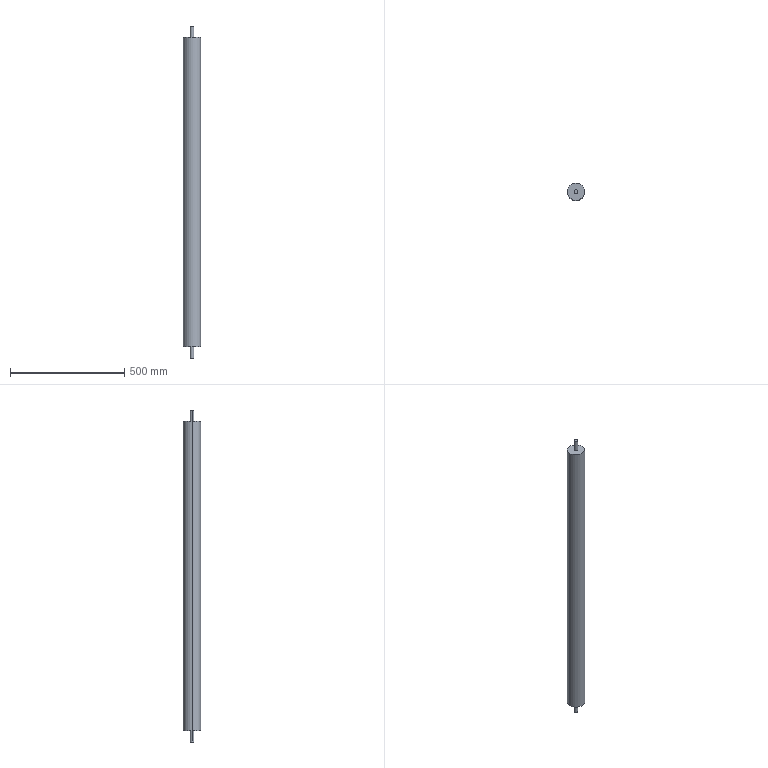Part | SolidWorks | features Extrusion 1, ICE 1, MirrorPattern 1 | 1 solid | 10 faces | box 76 x 76 x 1450 mm | volume 6144327 mm3 | cylinder 6 | plane 4 | commonest cylinder face diameters 16 x4 76 x2
STEP:
#1=CARTESIAN_POINT('',(8.,0.,-725.));
#2=VERTEX_POINT('',#1);
#3=CARTESIAN_POINT('',(-8.,0.,-725.));
#4=VERTEX_POINT('',#3);
#5=CARTESIAN_POINT('',(0.,0.,-725.));
#6=DIRECTION('',(0.,0.,1.));
#7=DIRECTION('',(1.,0.,0.));
#8=AXIS2_PLACEMENT_3D('',#5,#6,#7);
#9=CIRCLE('',#8,8.);
#10=EDGE_CURVE('',#2,#4,#9,.T.);
#11=ORIENTED_EDGE('',*,*,#10,.T.);
#12=CARTESIAN_POINT('',(-8.,0.,-675.));
#13=VERTEX_POINT('',#12);
#14=CARTESIAN_POINT('',(-8.,0.,-725.));
#15=DIRECTION('',(0.,0.,1.));
#16=VECTOR('',#15,1000.);
#17=LINE('',#14,#16);
#18=EDGE_CURVE('',#4,#13,#17,.T.);
#19=ORIENTED_EDGE('',*,*,#18,.T.);
#20=CARTESIAN_POINT('',(8.,0.,-675.));
#21=VERTEX_POINT('',#20);
#22=CARTESIAN_POINT('',(0.,0.,-675.));
#23=DIRECTION('',(0.,0.,1.));
#24=DIRECTION('',(1.,0.,0.));
#25=AXIS2_PLACEMENT_3D('',#22,#23,#24);
#26=CIRCLE('',#25,8.);
#27=EDGE_CURVE('',#21,#13,#26,.T.);
#28=ORIENTED_EDGE('',*,*,#27,.F.);
#29=CARTESIAN_POINT('',(8.,0.,-725.));
#30=DIRECTION('',(0.,0.,1.));
#31=VECTOR('',#30,1000.);
#32=LINE('',#29,#31);
#33=EDGE_CURVE('',#2,#21,#32,.T.);
#34=ORIENTED_EDGE('',*,*,#33,.F.);
#35=EDGE_LOOP('',(#11,#19,#28,#34));
#36=FACE_OUTER_BOUND('',#35,.T.);
#37=CARTESIAN_POINT('',(0.,0.,-725.));
#38=DIRECTION('',(0.,0.,1.));
#39=DIRECTION('',(1.,0.,0.));
#40=AXIS2_PLACEMENT_3D('',#37,#38,#39);
#41=CYLINDRICAL_SURFACE('',#40,8.);
#42=ADVANCED_FACE('',(#36),#41,.T.);
#43=CARTESIAN_POINT('',(8.,0.,725.));
#44=VERTEX_POINT('',#43);
#45=CARTESIAN_POINT('',(-8.,0.,725.));
#46=VERTEX_POINT('',#45);
#47=CARTESIAN_POINT('',(0.,0.,725.));
#48=DIRECTION('',(0.,0.,1.));
#49=DIRECTION('',(1.,0.,0.));
#50=AXIS2_PLACEMENT_3D('',#47,#48,#49);
#51=CIRCLE('',#50,8.);
#52=EDGE_CURVE('',#44,#46,#51,.T.);
#53=ORIENTED_EDGE('',*,*,#52,.F.);
#54=CARTESIAN_POINT('',(8.,0.,675.));
#55=VERTEX_POINT('',#54);
#56=CARTESIAN_POINT('',(8.,0.,725.));
#57=DIRECTION('',(0.,0.,-1.));
#58=VECTOR('',#57,1000.);
#59=LINE('',#56,#58);
#60=EDGE_CURVE('',#44,#55,#59,.T.);
#61=ORIENTED_EDGE('',*,*,#60,.T.);
#62=CARTESIAN_POINT('',(-8.,0.,675.));
#63=VERTEX_POINT('',#62);
#64=CARTESIAN_POINT('',(0.,0.,675.));
#65=DIRECTION('',(0.,0.,-1.));
#66=DIRECTION('',(1.,0.,0.));
#67=AXIS2_PLACEMENT_3D('',#64,#65,#66);
#68=CIRCLE('',#67,8.);
#69=EDGE_CURVE('',#63,#55,#68,.T.);
#70=ORIENTED_EDGE('',*,*,#69,.F.);
#71=CARTESIAN_POINT('',(-8.,0.,725.));
#72=DIRECTION('',(0.,0.,-1.));
#73=VECTOR('',#72,1000.);
#74=LINE('',#71,#73);
#75=EDGE_CURVE('',#46,#63,#74,.T.);
#76=ORIENTED_EDGE('',*,*,#75,.F.);
#77=EDGE_LOOP('',(#53,#61,#70,#76));
#78=FACE_OUTER_BOUND('',#77,.T.);
#79=CARTESIAN_POINT('',(0.,0.,725.));
#80=DIRECTION('',(0.,0.,-1.));
#81=DIRECTION('',(-1.,0.,0.));
#82=AXIS2_PLACEMENT_3D('',#79,#80,#81);
#83=CYLINDRICAL_SURFACE('',#82,8.);
#84=ADVANCED_FACE('',(#78),#83,.T.);
#85=CARTESIAN_POINT('',(38.,0.,675.));
#86=VERTEX_POINT('',#85);
#87=CARTESIAN_POINT('',(-38.,0.,675.));
#88=VERTEX_POINT('',#87);
#89=CARTESIAN_POINT('',(0.,0.,675.));
#90=DIRECTION('',(0.,0.,1.));
#91=DIRECTION('',(1.,0.,0.));
#92=AXIS2_PLACEMENT_3D('',#89,#90,#91);
#93=CIRCLE('',#92,38.);
#94=EDGE_CURVE('',#86,#88,#93,.T.);
#95=ORIENTED_EDGE('',*,*,#94,.F.);
#96=CARTESIAN_POINT('',(38.,0.,-675.));
#97=VERTEX_POINT('',#96);
#98=CARTESIAN_POINT('',(38.,0.,675.));
#99=DIRECTION('',(0.,0.,-1.));
#100=VECTOR('',#99,1000.);
#101=LINE('',#98,#100);
#102=EDGE_CURVE('',#86,#97,#101,.T.);
#103=ORIENTED_EDGE('',*,*,#102,.T.);
#104=CARTESIAN_POINT('',(-38.,0.,-675.));
#105=VERTEX_POINT('',#104);
#106=CARTESIAN_POINT('',(0.,0.,-675.));
#107=DIRECTION('',(0.,0.,1.));
#108=DIRECTION('',(1.,0.,0.));
#109=AXIS2_PLACEMENT_3D('',#106,#107,#108);
#110=CIRCLE('',#109,38.);
#111=EDGE_CURVE('',#97,#105,#110,.T.);
#112=ORIENTED_EDGE('',*,*,#111,.T.);
#113=CARTESIAN_POINT('',(-38.,0.,675.));
#114=DIRECTION('',(0.,0.,-1.));
#115=VECTOR('',#114,1000.);
#116=LINE('',#113,#115);
#117=EDGE_CURVE('',#88,#105,#116,.T.);
#118=ORIENTED_EDGE('',*,*,#117,.F.);
#119=EDGE_LOOP('',(#95,#103,#112,#118));
#120=FACE_OUTER_BOUND('',#119,.T.);
#121=CARTESIAN_POINT('',(0.,0.,675.));
#122=DIRECTION('',(0.,0.,-1.));
#123=DIRECTION('',(-1.,0.,0.));
#124=AXIS2_PLACEMENT_3D('',#121,#122,#123);
#125=CYLINDRICAL_SURFACE('',#124,38.);
#126=ADVANCED_FACE('',(#120),#125,.T.);
#127=ORIENTED_EDGE('',*,*,#102,.F.);
#128=CARTESIAN_POINT('',(0.,0.,675.));
#129=DIRECTION('',(0.,0.,1.));
#130=DIRECTION('',(1.,0.,0.));
#131=AXIS2_PLACEMENT_3D('',#128,#129,#130);
#132=CIRCLE('',#131,38.);
#133=EDGE_CURVE('',#88,#86,#132,.T.);
#134=ORIENTED_EDGE('',*,*,#133,.F.);
#135=ORIENTED_EDGE('',*,*,#117,.T.);
#136=CARTESIAN_POINT('',(0.,0.,-675.));
#137=DIRECTION('',(0.,0.,1.));
#138=DIRECTION('',(1.,0.,0.));
#139=AXIS2_PLACEMENT_3D('',#136,#137,#138);
#140=CIRCLE('',#139,38.);
#141=EDGE_CURVE('',#105,#97,#140,.T.);
#142=ORIENTED_EDGE('',*,*,#141,.T.);
#143=EDGE_LOOP('',(#127,#134,#135,#142));
#144=FACE_OUTER_BOUND('',#143,.T.);
#145=CARTESIAN_POINT('',(0.,0.,675.));
#146=DIRECTION('',(0.,0.,-1.));
#147=DIRECTION('',(-1.,0.,0.));
#148=AXIS2_PLACEMENT_3D('',#145,#146,#147);
#149=CYLINDRICAL_SURFACE('',#148,38.);
#150=ADVANCED_FACE('',(#144),#149,.T.);
#151=ORIENTED_EDGE('',*,*,#69,.T.);
#152=CARTESIAN_POINT('',(0.,0.,675.));
#153=DIRECTION('',(0.,0.,-1.));
#154=DIRECTION('',(1.,0.,0.));
#155=AXIS2_PLACEMENT_3D('',#152,#153,#154);
#156=CIRCLE('',#155,8.);
#157=EDGE_CURVE('',#55,#63,#156,.T.);
#158=ORIENTED_EDGE('',*,*,#157,.T.);
#159=EDGE_LOOP('',(#151,#158));
#160=FACE_BOUND('',#159,.T.);
#161=ORIENTED_EDGE('',*,*,#133,.T.);
#162=ORIENTED_EDGE('',*,*,#94,.T.);
#163=EDGE_LOOP('',(#161,#162));
#164=FACE_OUTER_BOUND('',#163,.T.);
#165=CARTESIAN_POINT('',(0.,0.,675.));
#166=DIRECTION('',(0.,0.,1.));
#167=DIRECTION('',(1.,0.,0.));
#168=AXIS2_PLACEMENT_3D('',#165,#166,#167);
#169=PLANE('',#168);
#170=ADVANCED_FACE('',(#160,#164),#169,.T.);
#171=ORIENTED_EDGE('',*,*,#27,.T.);
#172=CARTESIAN_POINT('',(0.,0.,-675.));
#173=DIRECTION('',(0.,0.,1.));
#174=DIRECTION('',(1.,0.,0.));
#175=AXIS2_PLACEMENT_3D('',#172,#173,#174);
#176=CIRCLE('',#175,8.);
#177=EDGE_CURVE('',#13,#21,#176,.T.);
#178=ORIENTED_EDGE('',*,*,#177,.T.);
#179=EDGE_LOOP('',(#171,#178));
#180=FACE_BOUND('',#179,.T.);
#181=ORIENTED_EDGE('',*,*,#141,.F.);
#182=ORIENTED_EDGE('',*,*,#111,.F.);
#183=EDGE_LOOP('',(#181,#182));
#184=FACE_OUTER_BOUND('',#183,.T.);
#185=CARTESIAN_POINT('',(0.,0.,-675.));
#186=DIRECTION('',(0.,0.,1.));
#187=DIRECTION('',(1.,0.,0.));
#188=AXIS2_PLACEMENT_3D('',#185,#186,#187);
#189=PLANE('',#188);
#190=ADVANCED_FACE('',(#180,#184),#189,.F.);
#191=ORIENTED_EDGE('',*,*,#60,.F.);
#192=CARTESIAN_POINT('',(0.,0.,725.));
#193=DIRECTION('',(0.,0.,1.));
#194=DIRECTION('',(1.,0.,0.));
#195=AXIS2_PLACEMENT_3D('',#192,#193,#194);
#196=CIRCLE('',#195,8.);
#197=EDGE_CURVE('',#46,#44,#196,.T.);
#198=ORIENTED_EDGE('',*,*,#197,.F.);
#199=ORIENTED_EDGE('',*,*,#75,.T.);
#200=ORIENTED_EDGE('',*,*,#157,.F.);
#201=EDGE_LOOP('',(#191,#198,#199,#200));
#202=FACE_OUTER_BOUND('',#201,.T.);
#203=CARTESIAN_POINT('',(0.,0.,725.));
#204=DIRECTION('',(0.,0.,-1.));
#205=DIRECTION('',(-1.,0.,0.));
#206=AXIS2_PLACEMENT_3D('',#203,#204,#205);
#207=CYLINDRICAL_SURFACE('',#206,8.);
#208=ADVANCED_FACE('',(#202),#207,.T.);
#209=ORIENTED_EDGE('',*,*,#197,.T.);
#210=ORIENTED_EDGE('',*,*,#52,.T.);
#211=EDGE_LOOP('',(#209,#210));
#212=FACE_OUTER_BOUND('',#211,.T.);
#213=CARTESIAN_POINT('',(0.,0.,725.));
#214=DIRECTION('',(0.,0.,1.));
#215=DIRECTION('',(1.,0.,0.));
#216=AXIS2_PLACEMENT_3D('',#213,#214,#215);
#217=PLANE('',#216);
#218=ADVANCED_FACE('',(#212),#217,.T.);
#219=ORIENTED_EDGE('',*,*,#18,.F.);
#220=CARTESIAN_POINT('',(0.,0.,-725.));
#221=DIRECTION('',(0.,0.,1.));
#222=DIRECTION('',(1.,0.,0.));
#223=AXIS2_PLACEMENT_3D('',#220,#221,#222);
#224=CIRCLE('',#223,8.);
#225=EDGE_CURVE('',#4,#2,#224,.T.);
#226=ORIENTED_EDGE('',*,*,#225,.T.);
#227=ORIENTED_EDGE('',*,*,#33,.T.);
#228=ORIENTED_EDGE('',*,*,#177,.F.);
#229=EDGE_LOOP('',(#219,#226,#227,#228));
#230=FACE_OUTER_BOUND('',#229,.T.);
#231=CARTESIAN_POINT('',(0.,0.,-725.));
#232=DIRECTION('',(0.,0.,1.));
#233=DIRECTION('',(1.,0.,0.));
#234=AXIS2_PLACEMENT_3D('',#231,#232,#233);
#235=CYLINDRICAL_SURFACE('',#234,8.);
#236=ADVANCED_FACE('',(#230),#235,.T.);
#237=ORIENTED_EDGE('',*,*,#10,.F.);
#238=ORIENTED_EDGE('',*,*,#225,.F.);
#239=EDGE_LOOP('',(#237,#238));
#240=FACE_OUTER_BOUND('',#239,.T.);
#241=CARTESIAN_POINT('',(0.,0.,-725.));
#242=DIRECTION('',(0.,0.,-1.));
#243=DIRECTION('',(1.,0.,0.));
#244=AXIS2_PLACEMENT_3D('',#241,#242,#243);
#245=PLANE('',#244);
#246=ADVANCED_FACE('',(#240),#245,.T.);
#247=CLOSED_SHELL('',(#42,#84,#126,#150,#170,#190,#208,#218,#236,#246));
#248=MANIFOLD_SOLID_BREP('',#247);
#249=CARTESIAN_POINT('',(0.,0.,0.));
#250=DIRECTION('',(0.,0.,1.));
#251=DIRECTION('',(1.,0.,0.));
#252=AXIS2_PLACEMENT_3D('',#249,#250,#251);
#253=(LENGTH_UNIT()NAMED_UNIT(*)SI_UNIT(.MILLI.,.METRE.));
#254=UNCERTAINTY_MEASURE_WITH_UNIT(LENGTH_MEASURE(0.00001),#253,'','');
#255=(NAMED_UNIT(*)PLANE_ANGLE_UNIT()SI_UNIT($,.RADIAN.));
#256=(NAMED_UNIT(*)SI_UNIT($,.STERADIAN.)SOLID_ANGLE_UNIT());
#257=(GEOMETRIC_REPRESENTATION_CONTEXT(3)GLOBAL_UNCERTAINTY_ASSIGNED_CONTEXT((#254))GLOBAL_UNIT_ASSIGNED_CONTEXT((#253,#255,#256))REPRESENTATION_CONTEXT('',''));
#258=ADVANCED_BREP_SHAPE_REPRESENTATION('',(#248,#252),#257);